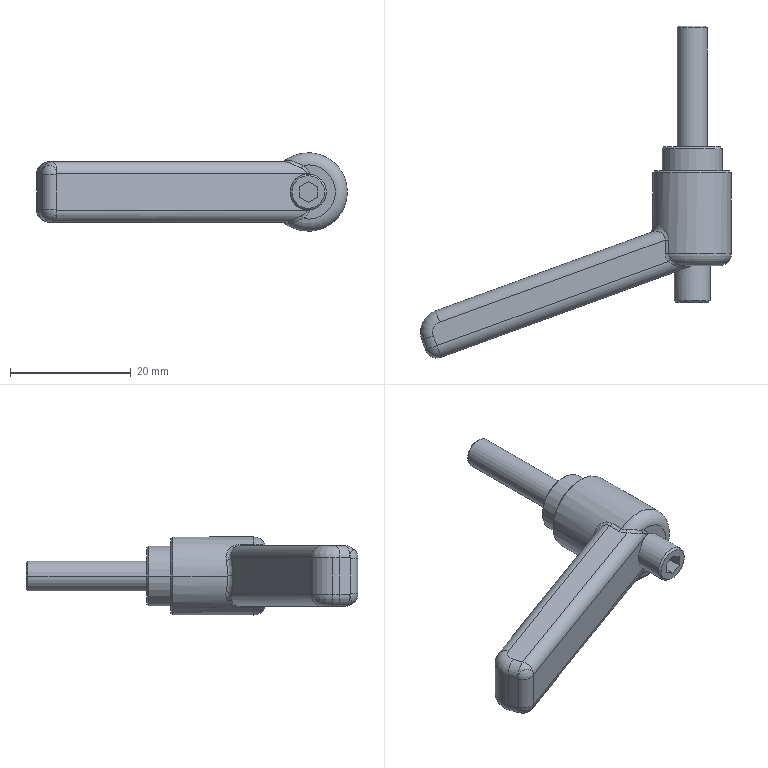Part | NX | 1 solid | 62 faces | box 51.5 x 55 x 13 mm | volume 5883 mm3 | cylinder 19 | plane 17 | spline 12 | cone 8 | torus 4 | sphere 2 | commonest cylinder face diameters 4 x6 2 x2 5 x2 6 x2 7.5 x2 10 x2